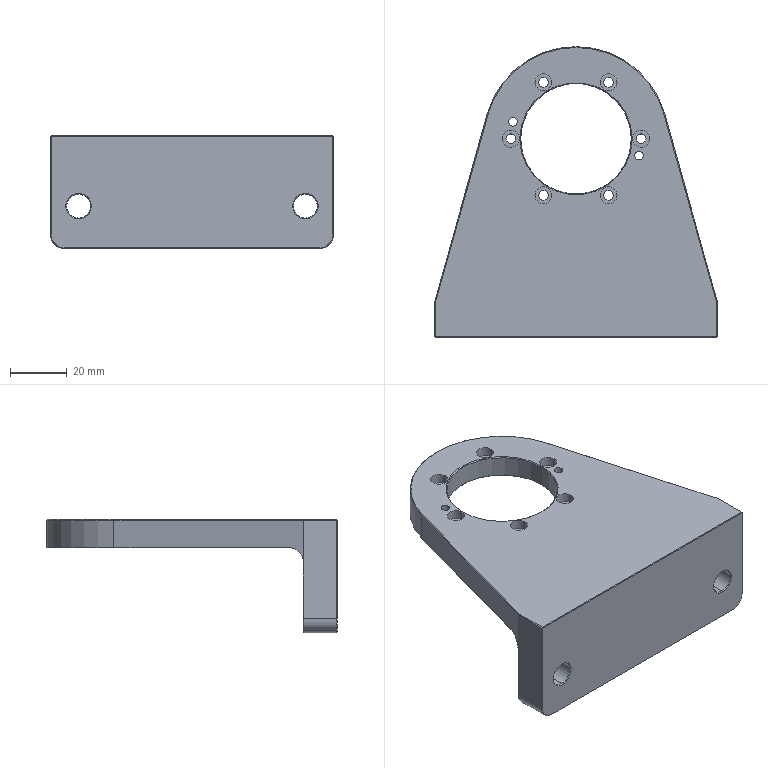NC program | NX | posted with a generic post | part box 100 x 102.5 x 40 mm
Whole program:
N10 G17 G21 G94 G90
(DRILLING_COPY_1_1 , TOOL : D6A45)
N12 T01 M6
N14 G54
N16 G17 G0 G90 X40. Y5. B0. C0. S5000 M3
N18 G43 Z30. H1
N20 G94 G81 G98 Z-1.8 F350. R3.
N22 X-40.
N24 G80
N26 G0 X-40. Y5. Z30.
N28 M5
(DRILLING_COPY_1_COPY_COPY , TOOL : 8.4ZT)
N30 T20 M6
N32 G54
N34 G17 G0 G90 X-40. Y5. B0. C0. S2000 M3
N36 G43 Z30. H20
N38 G94 G83 G98 Z-16.024 F100. Q2. R3.
N40 X40.
N42 G80
N44 G0 X40. Y5. Z30.
N46 M5
N48 M2